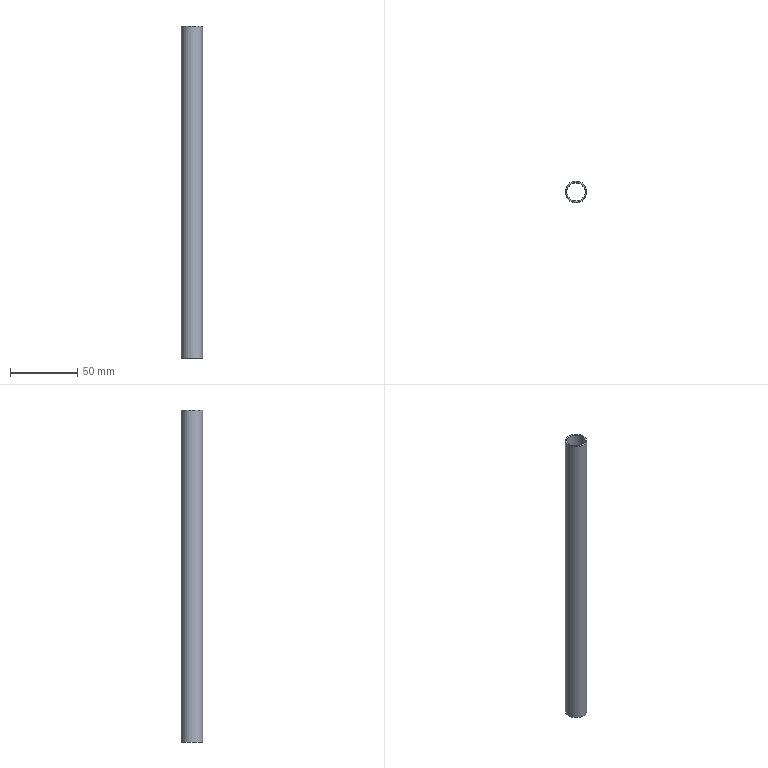Part | NX | features MG0313 aframe 2 | 1 solid | 4 faces | box 15.875 x 15.875 x 247.65 mm | volume 11745 mm3 | cylinder 2 | plane 2 | commonest cylinder face diameters 13.843 x1 15.875 x1
STEP:
#1=CARTESIAN_POINT('',(7.938,0.,123.825));
#2=VERTEX_POINT('',#1);
#3=CARTESIAN_POINT('',(0.,0.,123.825));
#4=DIRECTION('',(0.,0.,1.));
#5=DIRECTION('',(1.,0.,0.));
#6=AXIS2_PLACEMENT_3D('',#3,#4,#5);
#7=CIRCLE('',#6,7.938);
#8=EDGE_CURVE('',#2,#2,#7,.T.);
#9=ORIENTED_EDGE('',*,*,#8,.F.);
#10=EDGE_LOOP('',(#9));
#11=FACE_BOUND('',#10,.T.);
#12=CARTESIAN_POINT('',(7.938,0.,-123.825));
#13=VERTEX_POINT('',#12);
#14=CARTESIAN_POINT('',(0.,0.,-123.825));
#15=DIRECTION('',(0.,0.,1.));
#16=DIRECTION('',(1.,0.,0.));
#17=AXIS2_PLACEMENT_3D('',#14,#15,#16);
#18=CIRCLE('',#17,7.938);
#19=EDGE_CURVE('',#13,#13,#18,.T.);
#20=ORIENTED_EDGE('',*,*,#19,.T.);
#21=EDGE_LOOP('',(#20));
#22=FACE_BOUND('',#21,.T.);
#23=CARTESIAN_POINT('',(0.,0.,-123.825));
#24=DIRECTION('',(0.,0.,1.));
#25=DIRECTION('',(1.,0.,0.));
#26=AXIS2_PLACEMENT_3D('',#23,#24,#25);
#27=CYLINDRICAL_SURFACE('',#26,7.938);
#28=ADVANCED_FACE('',(#11,#22),#27,.T.);
#29=CARTESIAN_POINT('',(6.921,0.,-123.825));
#30=VERTEX_POINT('',#29);
#31=CARTESIAN_POINT('',(0.,0.,-123.825));
#32=DIRECTION('',(0.,0.,1.));
#33=DIRECTION('',(1.,0.,0.));
#34=AXIS2_PLACEMENT_3D('',#31,#32,#33);
#35=CIRCLE('',#34,6.921);
#36=EDGE_CURVE('',#30,#30,#35,.T.);
#37=ORIENTED_EDGE('',*,*,#36,.T.);
#38=EDGE_LOOP('',(#37));
#39=FACE_BOUND('',#38,.T.);
#40=ORIENTED_EDGE('',*,*,#19,.F.);
#41=EDGE_LOOP('',(#40));
#42=FACE_BOUND('',#41,.T.);
#43=CARTESIAN_POINT('',(0.,0.,-123.825));
#44=DIRECTION('',(0.,0.,1.));
#45=DIRECTION('',(1.,0.,0.));
#46=AXIS2_PLACEMENT_3D('',#43,#44,#45);
#47=PLANE('',#46);
#48=ADVANCED_FACE('',(#39,#42),#47,.F.);
#49=ORIENTED_EDGE('',*,*,#36,.F.);
#50=EDGE_LOOP('',(#49));
#51=FACE_BOUND('',#50,.T.);
#52=CARTESIAN_POINT('',(6.921,0.,123.825));
#53=VERTEX_POINT('',#52);
#54=CARTESIAN_POINT('',(0.,0.,123.825));
#55=DIRECTION('',(0.,0.,1.));
#56=DIRECTION('',(1.,0.,0.));
#57=AXIS2_PLACEMENT_3D('',#54,#55,#56);
#58=CIRCLE('',#57,6.921);
#59=EDGE_CURVE('',#53,#53,#58,.T.);
#60=ORIENTED_EDGE('',*,*,#59,.T.);
#61=EDGE_LOOP('',(#60));
#62=FACE_BOUND('',#61,.T.);
#63=CARTESIAN_POINT('',(0.,0.,-123.825));
#64=DIRECTION('',(0.,0.,1.));
#65=DIRECTION('',(1.,0.,0.));
#66=AXIS2_PLACEMENT_3D('',#63,#64,#65);
#67=CYLINDRICAL_SURFACE('',#66,6.921);
#68=ADVANCED_FACE('',(#51,#62),#67,.F.);
#69=ORIENTED_EDGE('',*,*,#8,.T.);
#70=EDGE_LOOP('',(#69));
#71=FACE_BOUND('',#70,.T.);
#72=ORIENTED_EDGE('',*,*,#59,.F.);
#73=EDGE_LOOP('',(#72));
#74=FACE_BOUND('',#73,.T.);
#75=CARTESIAN_POINT('',(0.,0.,123.825));
#76=DIRECTION('',(0.,0.,1.));
#77=DIRECTION('',(1.,0.,0.));
#78=AXIS2_PLACEMENT_3D('',#75,#76,#77);
#79=PLANE('',#78);
#80=ADVANCED_FACE('',(#71,#74),#79,.T.);
#81=CLOSED_SHELL('',(#28,#48,#68,#80));
#82=MANIFOLD_SOLID_BREP('',#81);
#83=(LENGTH_UNIT()NAMED_UNIT(*)SI_UNIT(.MILLI.,.METRE.));
#84=UNCERTAINTY_MEASURE_WITH_UNIT(LENGTH_MEASURE(0.00001),#83,'','');
#85=(NAMED_UNIT(*)PLANE_ANGLE_UNIT()SI_UNIT($,.RADIAN.));
#86=(NAMED_UNIT(*)SI_UNIT($,.STERADIAN.)SOLID_ANGLE_UNIT());
#87=(GEOMETRIC_REPRESENTATION_CONTEXT(3)GLOBAL_UNCERTAINTY_ASSIGNED_CONTEXT((#84))GLOBAL_UNIT_ASSIGNED_CONTEXT((#83,#85,#86))REPRESENTATION_CONTEXT('',''));
#88=ADVANCED_BREP_SHAPE_REPRESENTATION('',(#82),#87);